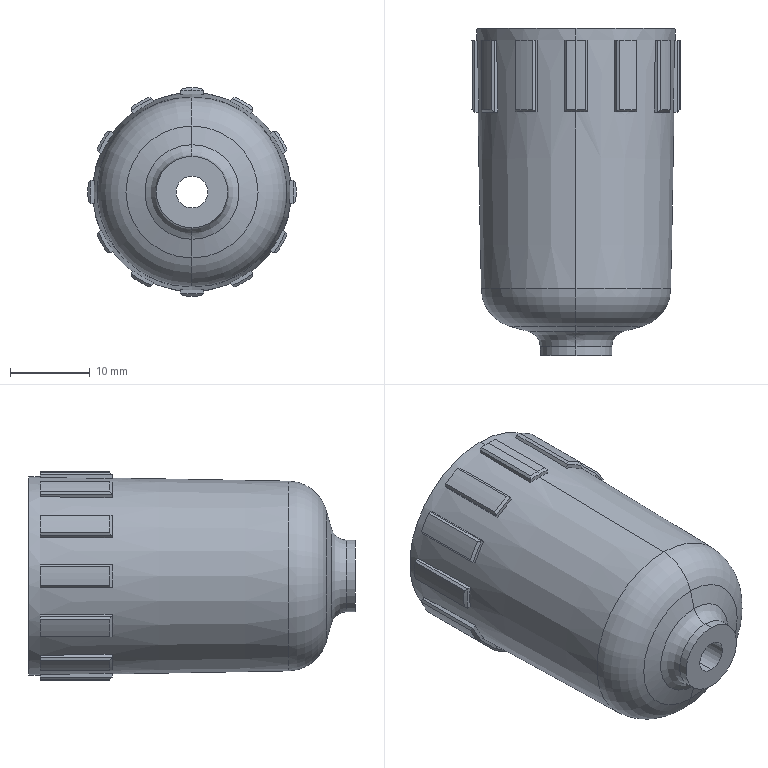Part | STEP file | AC10B-M5_AC3011A AF Bowl(10)-1 | 1 solid | 119 faces | box 26.2 x 41.1 x 26.2 mm | volume 3344 mm3 | plane 75 | cone 21 | cylinder 17 | torus 6 | commonest cylinder face diameters 26.2 x13 4 x2 9 x2